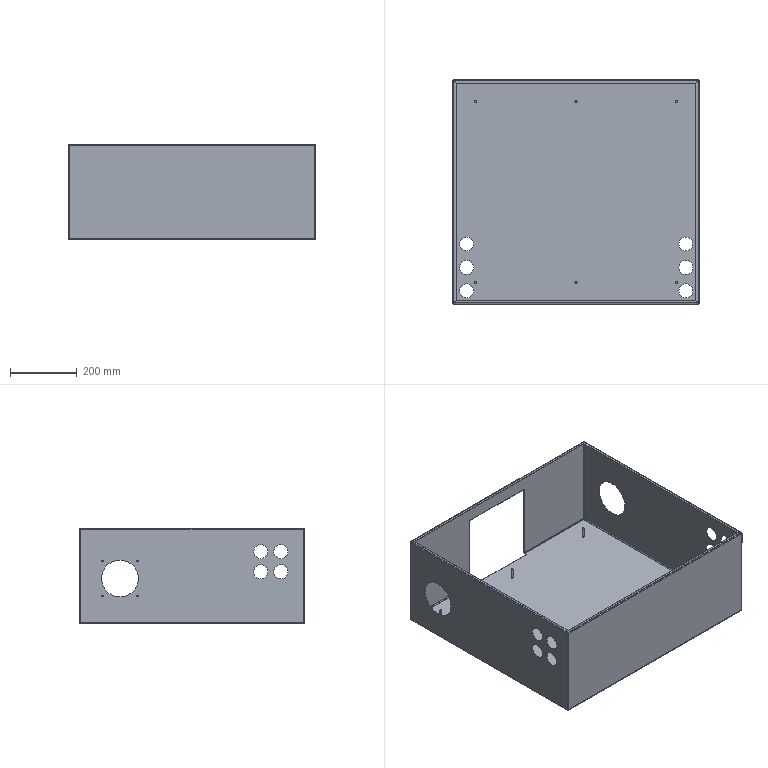Part | SolidWorks | features ICE 5, EdgeFlange 2, FlatPattern 1, LPattern 1, SMBaseFlange 1, SheetMetal 1 | 1 solid | 146 faces | box 736 x 670 x 285 mm | volume 1816842 mm3 | cylinder 78 | plane 52 | spline 16 | commonest cylinder face diameters 42 x28 5 x16 6 x12 4 x9 7 x9 110 x4